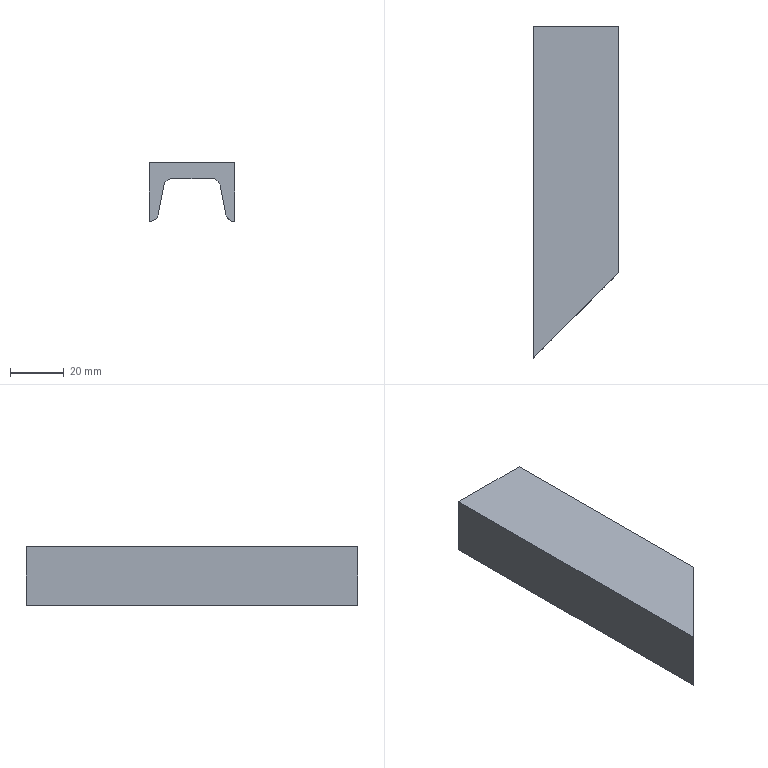Part | NX | features solid 2 | 1 solid | 14 faces | box 32 x 124.084 x 22 mm | volume 35993 mm3 | plane 10 | cylinder 4 | commonest cylinder face diameters 6 x4
STEP:
#1=CARTESIAN_POINT('',(-60.648,443.3,62.866));
#2=VERTEX_POINT('',#1);
#3=CARTESIAN_POINT('',(-60.648,319.567,62.866));
#4=VERTEX_POINT('',#3);
#5=CARTESIAN_POINT('',(-60.648,367.216,62.866));
#6=DIRECTION('',(0.,1.,0.));
#7=VECTOR('',#6,1000.);
#8=LINE('',#5,#7);
#9=EDGE_CURVE('',#2,#4,#8,.F.);
#10=ORIENTED_EDGE('',*,*,#9,.T.);
#11=CARTESIAN_POINT('',(-61.,319.216,62.866));
#12=VERTEX_POINT('',#11);
#13=CARTESIAN_POINT('',(-22.5,357.716,62.866));
#14=DIRECTION('',(-0.7071,-0.7071,0.));
#15=VECTOR('',#14,1000.);
#16=LINE('',#13,#15);
#17=EDGE_CURVE('',#4,#12,#16,.T.);
#18=ORIENTED_EDGE('',*,*,#17,.T.);
#19=CARTESIAN_POINT('',(-61.,443.3,62.866));
#20=VERTEX_POINT('',#19);
#21=CARTESIAN_POINT('',(-61.,380.216,62.866));
#22=DIRECTION('',(0.,1.,0.));
#23=VECTOR('',#22,1000.);
#24=LINE('',#21,#23);
#25=EDGE_CURVE('',#20,#12,#24,.F.);
#26=ORIENTED_EDGE('',*,*,#25,.F.);
#27=CARTESIAN_POINT('',(-67.,443.3,62.866));
#28=DIRECTION('',(-1.,0.,0.));
#29=VECTOR('',#28,1000.);
#30=LINE('',#27,#29);
#31=EDGE_CURVE('',#2,#20,#30,.T.);
#32=ORIENTED_EDGE('',*,*,#31,.F.);
#33=EDGE_LOOP('',(#10,#18,#26,#32));
#34=FACE_BOUND('',#33,.T.);
#35=CARTESIAN_POINT('',(-45.,380.216,62.866));
#36=DIRECTION('',(0.,0.,-1.));
#37=DIRECTION('',(0.,-1.,0.));
#38=AXIS2_PLACEMENT_3D('',#35,#36,#37);
#39=PLANE('',#38);
#40=ADVANCED_FACE('',(#34),#39,.T.);
#41=CARTESIAN_POINT('',(-29.,351.216,62.866));
#42=VERTEX_POINT('',#41);
#43=CARTESIAN_POINT('',(-29.,443.3,62.866));
#44=VERTEX_POINT('',#43);
#45=CARTESIAN_POINT('',(-29.,380.216,62.866));
#46=DIRECTION('',(0.,-1.,0.));
#47=VECTOR('',#46,1000.);
#48=LINE('',#45,#47);
#49=EDGE_CURVE('',#42,#44,#48,.F.);
#50=ORIENTED_EDGE('',*,*,#49,.F.);
#51=CARTESIAN_POINT('',(-29.352,350.864,62.866));
#52=VERTEX_POINT('',#51);
#53=CARTESIAN_POINT('',(-22.5,357.716,62.866));
#54=DIRECTION('',(-0.7071,-0.7071,0.));
#55=VECTOR('',#54,1000.);
#56=LINE('',#53,#55);
#57=EDGE_CURVE('',#42,#52,#56,.T.);
#58=ORIENTED_EDGE('',*,*,#57,.T.);
#59=CARTESIAN_POINT('',(-29.352,443.3,62.866));
#60=VERTEX_POINT('',#59);
#61=CARTESIAN_POINT('',(-29.352,380.216,62.866));
#62=DIRECTION('',(0.,1.,0.));
#63=VECTOR('',#62,1000.);
#64=LINE('',#61,#63);
#65=EDGE_CURVE('',#52,#60,#64,.T.);
#66=ORIENTED_EDGE('',*,*,#65,.T.);
#67=CARTESIAN_POINT('',(-67.,443.3,62.866));
#68=DIRECTION('',(-1.,0.,0.));
#69=VECTOR('',#68,1000.);
#70=LINE('',#67,#69);
#71=EDGE_CURVE('',#44,#60,#70,.T.);
#72=ORIENTED_EDGE('',*,*,#71,.F.);
#73=EDGE_LOOP('',(#50,#58,#66,#72));
#74=FACE_BOUND('',#73,.T.);
#75=CARTESIAN_POINT('',(-45.,380.216,62.866));
#76=DIRECTION('',(0.,0.,-1.));
#77=DIRECTION('',(0.,-1.,0.));
#78=AXIS2_PLACEMENT_3D('',#75,#76,#77);
#79=PLANE('',#78);
#80=ADVANCED_FACE('',(#74),#79,.T.);
#81=CARTESIAN_POINT('',(-61.,319.216,84.866));
#82=VERTEX_POINT('',#81);
#83=CARTESIAN_POINT('',(-61.,443.3,84.866));
#84=VERTEX_POINT('',#83);
#85=CARTESIAN_POINT('',(-61.,380.216,84.866));
#86=DIRECTION('',(0.,-1.,0.));
#87=VECTOR('',#86,1000.);
#88=LINE('',#85,#87);
#89=EDGE_CURVE('',#82,#84,#88,.F.);
#90=ORIENTED_EDGE('',*,*,#89,.F.);
#91=CARTESIAN_POINT('',(-29.,351.216,84.866));
#92=VERTEX_POINT('',#91);
#93=CARTESIAN_POINT('',(-22.5,357.716,84.866));
#94=DIRECTION('',(0.7071,0.7071,0.));
#95=VECTOR('',#94,1000.);
#96=LINE('',#93,#95);
#97=EDGE_CURVE('',#82,#92,#96,.T.);
#98=ORIENTED_EDGE('',*,*,#97,.T.);
#99=CARTESIAN_POINT('',(-29.,443.3,84.866));
#100=VERTEX_POINT('',#99);
#101=CARTESIAN_POINT('',(-29.,380.216,84.866));
#102=DIRECTION('',(0.,1.,0.));
#103=VECTOR('',#102,1000.);
#104=LINE('',#101,#103);
#105=EDGE_CURVE('',#100,#92,#104,.F.);
#106=ORIENTED_EDGE('',*,*,#105,.F.);
#107=CARTESIAN_POINT('',(-67.,443.3,84.866));
#108=DIRECTION('',(1.,0.,0.));
#109=VECTOR('',#108,1000.);
#110=LINE('',#107,#109);
#111=EDGE_CURVE('',#84,#100,#110,.T.);
#112=ORIENTED_EDGE('',*,*,#111,.F.);
#113=EDGE_LOOP('',(#90,#98,#106,#112));
#114=FACE_BOUND('',#113,.T.);
#115=CARTESIAN_POINT('',(-45.,380.216,84.866));
#116=DIRECTION('',(0.,0.,1.));
#117=DIRECTION('',(0.,1.,0.));
#118=AXIS2_PLACEMENT_3D('',#115,#116,#117);
#119=PLANE('',#118);
#120=ADVANCED_FACE('',(#114),#119,.T.);
#121=ORIENTED_EDGE('',*,*,#105,.T.);
#122=CARTESIAN_POINT('',(-29.,351.216,74.866));
#123=DIRECTION('',(0.,0.,-1.));
#124=VECTOR('',#123,1000.);
#125=LINE('',#122,#124);
#126=EDGE_CURVE('',#92,#42,#125,.T.);
#127=ORIENTED_EDGE('',*,*,#126,.T.);
#128=ORIENTED_EDGE('',*,*,#49,.T.);
#129=CARTESIAN_POINT('',(-29.,443.3,84.));
#130=DIRECTION('',(0.,0.,-1.));
#131=VECTOR('',#130,1000.);
#132=LINE('',#129,#131);
#133=EDGE_CURVE('',#100,#44,#132,.T.);
#134=ORIENTED_EDGE('',*,*,#133,.F.);
#135=EDGE_LOOP('',(#121,#127,#128,#134));
#136=FACE_BOUND('',#135,.T.);
#137=CARTESIAN_POINT('',(-29.,380.216,74.866));
#138=DIRECTION('',(1.,0.,0.));
#139=DIRECTION('',(0.,0.,1.));
#140=AXIS2_PLACEMENT_3D('',#137,#138,#139);
#141=PLANE('',#140);
#142=ADVANCED_FACE('',(#136),#141,.T.);
#143=CARTESIAN_POINT('',(-52.539,327.677,78.866));
#144=VERTEX_POINT('',#143);
#145=CARTESIAN_POINT('',(-37.461,342.754,78.866));
#146=VERTEX_POINT('',#145);
#147=CARTESIAN_POINT('',(-22.5,357.716,78.866));
#148=DIRECTION('',(0.7071,0.7071,0.));
#149=VECTOR('',#148,1000.);
#150=LINE('',#147,#149);
#151=EDGE_CURVE('',#144,#146,#150,.T.);
#152=ORIENTED_EDGE('',*,*,#151,.F.);
#153=CARTESIAN_POINT('',(-52.539,443.3,78.866));
#154=VERTEX_POINT('',#153);
#155=CARTESIAN_POINT('',(-52.539,319.216,78.866));
#156=DIRECTION('',(0.,-1.,0.));
#157=VECTOR('',#156,1000.);
#158=LINE('',#155,#157);
#159=EDGE_CURVE('',#144,#154,#158,.F.);
#160=ORIENTED_EDGE('',*,*,#159,.T.);
#161=CARTESIAN_POINT('',(-37.461,443.3,78.866));
#162=VERTEX_POINT('',#161);
#163=CARTESIAN_POINT('',(-67.,443.3,78.866));
#164=DIRECTION('',(1.,0.,0.));
#165=VECTOR('',#164,1000.);
#166=LINE('',#163,#165);
#167=EDGE_CURVE('',#154,#162,#166,.T.);
#168=ORIENTED_EDGE('',*,*,#167,.T.);
#169=CARTESIAN_POINT('',(-37.461,415.216,78.866));
#170=DIRECTION('',(0.,1.,0.));
#171=VECTOR('',#170,1000.);
#172=LINE('',#169,#171);
#173=EDGE_CURVE('',#162,#146,#172,.F.);
#174=ORIENTED_EDGE('',*,*,#173,.T.);
#175=EDGE_LOOP('',(#152,#160,#168,#174));
#176=FACE_BOUND('',#175,.T.);
#177=CARTESIAN_POINT('',(-45.,380.216,78.866));
#178=DIRECTION('',(0.,0.,1.));
#179=DIRECTION('',(0.,1.,0.));
#180=AXIS2_PLACEMENT_3D('',#177,#178,#179);
#181=PLANE('',#180);
#182=ADVANCED_FACE('',(#176),#181,.F.);
#183=CARTESIAN_POINT('',(-57.706,322.51,65.28));
#184=VERTEX_POINT('',#183);
#185=CARTESIAN_POINT('',(-55.481,324.735,76.452));
#186=VERTEX_POINT('',#185);
#187=CARTESIAN_POINT('',(-55.726,324.49,75.222));
#188=DIRECTION('',(0.1917,0.1917,0.9625));
#189=VECTOR('',#188,1000.);
#190=LINE('',#187,#189);
#191=EDGE_CURVE('',#184,#186,#190,.T.);
#192=ORIENTED_EDGE('',*,*,#191,.F.);
#193=CARTESIAN_POINT('',(-57.706,443.3,65.28));
#194=VERTEX_POINT('',#193);
#195=CARTESIAN_POINT('',(-57.706,367.216,65.28));
#196=DIRECTION('',(0.,1.,0.));
#197=VECTOR('',#196,1000.);
#198=LINE('',#195,#197);
#199=EDGE_CURVE('',#184,#194,#198,.T.);
#200=ORIENTED_EDGE('',*,*,#199,.T.);
#201=CARTESIAN_POINT('',(-55.481,443.3,76.452));
#202=VERTEX_POINT('',#201);
#203=CARTESIAN_POINT('',(-57.356,443.3,67.036));
#204=DIRECTION('',(-0.1953,0.,-0.9807));
#205=VECTOR('',#204,1000.);
#206=LINE('',#203,#205);
#207=EDGE_CURVE('',#202,#194,#206,.T.);
#208=ORIENTED_EDGE('',*,*,#207,.F.);
#209=CARTESIAN_POINT('',(-55.481,380.216,76.452));
#210=DIRECTION('',(0.,-1.,0.));
#211=VECTOR('',#210,1000.);
#212=LINE('',#209,#211);
#213=EDGE_CURVE('',#202,#186,#212,.T.);
#214=ORIENTED_EDGE('',*,*,#213,.T.);
#215=EDGE_LOOP('',(#192,#200,#208,#214));
#216=FACE_BOUND('',#215,.T.);
#217=CARTESIAN_POINT('',(-57.356,367.216,67.036));
#218=DIRECTION('',(-0.9807,0.,0.1953));
#219=DIRECTION('',(-0.1953,0.,-0.9807));
#220=AXIS2_PLACEMENT_3D('',#217,#218,#219);
#221=PLANE('',#220);
#222=ADVANCED_FACE('',(#216),#221,.F.);
#223=CARTESIAN_POINT('',(-34.519,345.697,76.452));
#224=VERTEX_POINT('',#223);
#225=CARTESIAN_POINT('',(-32.294,347.922,65.28));
#226=VERTEX_POINT('',#225);
#227=CARTESIAN_POINT('',(-31.922,348.294,63.411));
#228=DIRECTION('',(0.1917,0.1917,-0.9625));
#229=VECTOR('',#228,1000.);
#230=LINE('',#227,#229);
#231=EDGE_CURVE('',#224,#226,#230,.T.);
#232=ORIENTED_EDGE('',*,*,#231,.F.);
#233=CARTESIAN_POINT('',(-34.519,443.3,76.452));
#234=VERTEX_POINT('',#233);
#235=CARTESIAN_POINT('',(-34.519,380.216,76.452));
#236=DIRECTION('',(0.,1.,0.));
#237=VECTOR('',#236,1000.);
#238=LINE('',#235,#237);
#239=EDGE_CURVE('',#224,#234,#238,.T.);
#240=ORIENTED_EDGE('',*,*,#239,.T.);
#241=CARTESIAN_POINT('',(-32.294,443.3,65.28));
#242=VERTEX_POINT('',#241);
#243=CARTESIAN_POINT('',(-36.777,443.3,87.786));
#244=DIRECTION('',(0.1953,0.,-0.9807));
#245=VECTOR('',#244,1000.);
#246=LINE('',#243,#245);
#247=EDGE_CURVE('',#234,#242,#246,.T.);
#248=ORIENTED_EDGE('',*,*,#247,.T.);
#249=CARTESIAN_POINT('',(-32.294,380.216,65.28));
#250=DIRECTION('',(0.,1.,0.));
#251=VECTOR('',#250,1000.);
#252=LINE('',#249,#251);
#253=EDGE_CURVE('',#242,#226,#252,.F.);
#254=ORIENTED_EDGE('',*,*,#253,.T.);
#255=EDGE_LOOP('',(#232,#240,#248,#254));
#256=FACE_BOUND('',#255,.T.);
#257=CARTESIAN_POINT('',(-32.644,367.216,67.036));
#258=DIRECTION('',(0.9807,0.,0.1953));
#259=DIRECTION('',(-0.1953,0.,0.9807));
#260=AXIS2_PLACEMENT_3D('',#257,#258,#259);
#261=PLANE('',#260);
#262=ADVANCED_FACE('',(#256),#261,.F.);
#263=ORIENTED_EDGE('',*,*,#199,.F.);
#264=CARTESIAN_POINT('',(-60.648,319.567,65.866));
#265=DIRECTION('',(0.7071,-0.7071,0.));
#266=DIRECTION('',(-0.7071,-0.7071,0.));
#267=AXIS2_PLACEMENT_3D('',#264,#265,#266);
#268=ELLIPSE('',#267,4.243,3.);
#269=EDGE_CURVE('',#184,#4,#268,.F.);
#270=ORIENTED_EDGE('',*,*,#269,.T.);
#271=ORIENTED_EDGE('',*,*,#9,.F.);
#272=CARTESIAN_POINT('',(-60.648,443.3,65.866));
#273=DIRECTION('',(0.,1.,0.));
#274=DIRECTION('',(0.,0.,1.));
#275=AXIS2_PLACEMENT_3D('',#272,#273,#274);
#276=CIRCLE('',#275,3.);
#277=EDGE_CURVE('',#194,#2,#276,.T.);
#278=ORIENTED_EDGE('',*,*,#277,.F.);
#279=EDGE_LOOP('',(#263,#270,#271,#278));
#280=FACE_BOUND('',#279,.T.);
#281=CARTESIAN_POINT('',(-60.648,367.216,65.866));
#282=DIRECTION('',(0.,-1.,0.));
#283=DIRECTION('',(1.,0.,0.));
#284=AXIS2_PLACEMENT_3D('',#281,#282,#283);
#285=CYLINDRICAL_SURFACE('',#284,3.);
#286=ADVANCED_FACE('',(#280),#285,.T.);
#287=ORIENTED_EDGE('',*,*,#65,.F.);
#288=CARTESIAN_POINT('',(-29.352,350.864,65.866));
#289=DIRECTION('',(0.7071,-0.7071,0.));
#290=DIRECTION('',(-0.7071,-0.7071,0.));
#291=AXIS2_PLACEMENT_3D('',#288,#289,#290);
#292=ELLIPSE('',#291,4.243,3.);
#293=EDGE_CURVE('',#52,#226,#292,.F.);
#294=ORIENTED_EDGE('',*,*,#293,.T.);
#295=ORIENTED_EDGE('',*,*,#253,.F.);
#296=CARTESIAN_POINT('',(-29.352,443.3,65.866));
#297=DIRECTION('',(0.,1.,0.));
#298=DIRECTION('',(0.,0.,1.));
#299=AXIS2_PLACEMENT_3D('',#296,#297,#298);
#300=CIRCLE('',#299,3.);
#301=EDGE_CURVE('',#60,#242,#300,.T.);
#302=ORIENTED_EDGE('',*,*,#301,.F.);
#303=EDGE_LOOP('',(#287,#294,#295,#302));
#304=FACE_BOUND('',#303,.T.);
#305=CARTESIAN_POINT('',(-29.352,380.216,65.866));
#306=DIRECTION('',(0.,-1.,0.));
#307=DIRECTION('',(1.,0.,0.));
#308=AXIS2_PLACEMENT_3D('',#305,#306,#307);
#309=CYLINDRICAL_SURFACE('',#308,3.);
#310=ADVANCED_FACE('',(#304),#309,.T.);
#311=CARTESIAN_POINT('',(-37.461,342.754,75.866));
#312=DIRECTION('',(0.7071,-0.7071,0.));
#313=DIRECTION('',(-0.7071,-0.7071,0.));
#314=AXIS2_PLACEMENT_3D('',#311,#312,#313);
#315=ELLIPSE('',#314,4.243,3.);
#316=EDGE_CURVE('',#146,#224,#315,.F.);
#317=ORIENTED_EDGE('',*,*,#316,.F.);
#318=ORIENTED_EDGE('',*,*,#173,.F.);
#319=CARTESIAN_POINT('',(-37.461,443.3,75.866));
#320=DIRECTION('',(0.,1.,0.));
#321=DIRECTION('',(0.,0.,1.));
#322=AXIS2_PLACEMENT_3D('',#319,#320,#321);
#323=CIRCLE('',#322,3.);
#324=EDGE_CURVE('',#234,#162,#323,.F.);
#325=ORIENTED_EDGE('',*,*,#324,.F.);
#326=ORIENTED_EDGE('',*,*,#239,.F.);
#327=EDGE_LOOP('',(#317,#318,#325,#326));
#328=FACE_BOUND('',#327,.T.);
#329=CARTESIAN_POINT('',(-37.461,380.216,75.866));
#330=DIRECTION('',(0.,-1.,0.));
#331=DIRECTION('',(-1.,0.,0.));
#332=AXIS2_PLACEMENT_3D('',#329,#330,#331);
#333=CYLINDRICAL_SURFACE('',#332,3.);
#334=ADVANCED_FACE('',(#328),#333,.F.);
#335=CARTESIAN_POINT('',(-52.539,327.677,75.866));
#336=DIRECTION('',(0.7071,-0.7071,0.));
#337=DIRECTION('',(0.7071,0.7071,0.));
#338=AXIS2_PLACEMENT_3D('',#335,#336,#337);
#339=ELLIPSE('',#338,4.243,3.);
#340=EDGE_CURVE('',#186,#144,#339,.F.);
#341=ORIENTED_EDGE('',*,*,#340,.F.);
#342=ORIENTED_EDGE('',*,*,#213,.F.);
#343=CARTESIAN_POINT('',(-52.539,443.3,75.866));
#344=DIRECTION('',(0.,1.,0.));
#345=DIRECTION('',(0.,0.,1.));
#346=AXIS2_PLACEMENT_3D('',#343,#344,#345);
#347=CIRCLE('',#346,3.);
#348=EDGE_CURVE('',#154,#202,#347,.F.);
#349=ORIENTED_EDGE('',*,*,#348,.F.);
#350=ORIENTED_EDGE('',*,*,#159,.F.);
#351=EDGE_LOOP('',(#341,#342,#349,#350));
#352=FACE_BOUND('',#351,.T.);
#353=CARTESIAN_POINT('',(-52.539,380.216,75.866));
#354=DIRECTION('',(0.,1.,0.));
#355=DIRECTION('',(1.,0.,0.));
#356=AXIS2_PLACEMENT_3D('',#353,#354,#355);
#357=CYLINDRICAL_SURFACE('',#356,3.);
#358=ADVANCED_FACE('',(#352),#357,.F.);
#359=CARTESIAN_POINT('',(-61.,443.3,74.866));
#360=DIRECTION('',(0.,0.,-1.));
#361=VECTOR('',#360,1000.);
#362=LINE('',#359,#361);
#363=EDGE_CURVE('',#84,#20,#362,.T.);
#364=ORIENTED_EDGE('',*,*,#363,.T.);
#365=ORIENTED_EDGE('',*,*,#25,.T.);
#366=CARTESIAN_POINT('',(-61.,319.216,84.));
#367=DIRECTION('',(0.,0.,-1.));
#368=VECTOR('',#367,1000.);
#369=LINE('',#366,#368);
#370=EDGE_CURVE('',#82,#12,#369,.T.);
#371=ORIENTED_EDGE('',*,*,#370,.F.);
#372=ORIENTED_EDGE('',*,*,#89,.T.);
#373=EDGE_LOOP('',(#364,#365,#371,#372));
#374=FACE_BOUND('',#373,.T.);
#375=CARTESIAN_POINT('',(-61.,380.216,74.866));
#376=DIRECTION('',(-1.,0.,0.));
#377=DIRECTION('',(0.,0.,-1.));
#378=AXIS2_PLACEMENT_3D('',#375,#376,#377);
#379=PLANE('',#378);
#380=ADVANCED_FACE('',(#374),#379,.T.);
#381=ORIENTED_EDGE('',*,*,#31,.T.);
#382=ORIENTED_EDGE('',*,*,#363,.F.);
#383=ORIENTED_EDGE('',*,*,#111,.T.);
#384=ORIENTED_EDGE('',*,*,#133,.T.);
#385=ORIENTED_EDGE('',*,*,#71,.T.);
#386=ORIENTED_EDGE('',*,*,#301,.T.);
#387=ORIENTED_EDGE('',*,*,#247,.F.);
#388=ORIENTED_EDGE('',*,*,#324,.T.);
#389=ORIENTED_EDGE('',*,*,#167,.F.);
#390=ORIENTED_EDGE('',*,*,#348,.T.);
#391=ORIENTED_EDGE('',*,*,#207,.T.);
#392=ORIENTED_EDGE('',*,*,#277,.T.);
#393=EDGE_LOOP('',(#381,#382,#383,#384,#385,#386,#387,#388,#389,#390,#391,#392));
#394=FACE_BOUND('',#393,.T.);
#395=CARTESIAN_POINT('',(-67.,443.3,84.));
#396=DIRECTION('',(0.,1.,0.));
#397=DIRECTION('',(0.,0.,1.));
#398=AXIS2_PLACEMENT_3D('',#395,#396,#397);
#399=PLANE('',#398);
#400=ADVANCED_FACE('',(#394),#399,.T.);
#401=ORIENTED_EDGE('',*,*,#97,.F.);
#402=ORIENTED_EDGE('',*,*,#370,.T.);
#403=ORIENTED_EDGE('',*,*,#17,.F.);
#404=ORIENTED_EDGE('',*,*,#269,.F.);
#405=ORIENTED_EDGE('',*,*,#191,.T.);
#406=ORIENTED_EDGE('',*,*,#340,.T.);
#407=ORIENTED_EDGE('',*,*,#151,.T.);
#408=ORIENTED_EDGE('',*,*,#316,.T.);
#409=ORIENTED_EDGE('',*,*,#231,.T.);
#410=ORIENTED_EDGE('',*,*,#293,.F.);
#411=ORIENTED_EDGE('',*,*,#57,.F.);
#412=ORIENTED_EDGE('',*,*,#126,.F.);
#413=EDGE_LOOP('',(#401,#402,#403,#404,#405,#406,#407,#408,#409,#410,#411,#412));
#414=FACE_BOUND('',#413,.T.);
#415=CARTESIAN_POINT('',(-29.,351.216,0.5));
#416=DIRECTION('',(0.7071,-0.7071,0.));
#417=DIRECTION('',(0.7071,0.7071,0.));
#418=AXIS2_PLACEMENT_3D('',#415,#416,#417);
#419=PLANE('',#418);
#420=ADVANCED_FACE('',(#414),#419,.T.);
#421=CLOSED_SHELL('',(#40,#80,#120,#142,#182,#222,#262,#286,#310,#334,#358,#380,#400,#420));
#422=MANIFOLD_SOLID_BREP('',#421);
#423=(LENGTH_UNIT()NAMED_UNIT(*)SI_UNIT(.MILLI.,.METRE.));
#424=UNCERTAINTY_MEASURE_WITH_UNIT(LENGTH_MEASURE(0.00001),#423,'','');
#425=(NAMED_UNIT(*)PLANE_ANGLE_UNIT()SI_UNIT($,.RADIAN.));
#426=(NAMED_UNIT(*)SI_UNIT($,.STERADIAN.)SOLID_ANGLE_UNIT());
#427=(GEOMETRIC_REPRESENTATION_CONTEXT(3)GLOBAL_UNCERTAINTY_ASSIGNED_CONTEXT((#424))GLOBAL_UNIT_ASSIGNED_CONTEXT((#423,#425,#426))REPRESENTATION_CONTEXT('',''));
#428=ADVANCED_BREP_SHAPE_REPRESENTATION('',(#422),#427);